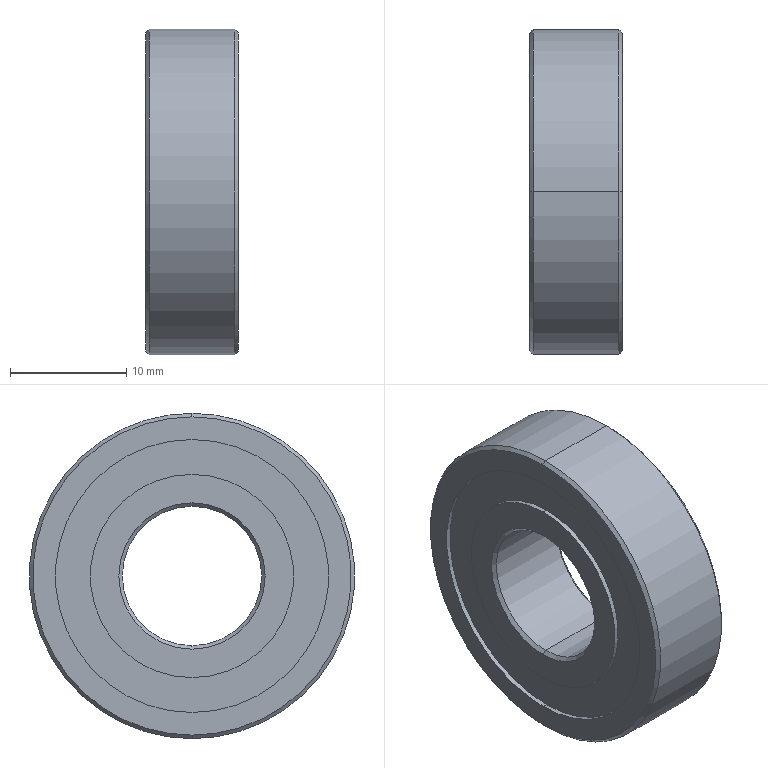Part | SolidWorks | features RefAxis 3, 3DProfileFeature 1, Revolution 1 | 1 solid | 26 faces | box 8 x 28 x 28 mm | volume 3855 mm3 | cylinder 12 | cone 8 | plane 6 | commonest cylinder face diameters 17.5 x4 23.5 x4 12 x2 28 x2
STEP:
#1=CARTESIAN_POINT('',(3.7,0.,14.));
#2=VERTEX_POINT('',#1);
#3=CARTESIAN_POINT('',(3.7,0.,-14.));
#4=VERTEX_POINT('',#3);
#5=CARTESIAN_POINT('',(3.7,0.,0.));
#6=DIRECTION('',(-1.,0.,0.));
#7=DIRECTION('',(0.,0.,1.));
#8=AXIS2_PLACEMENT_3D('',#5,#6,#7);
#9=CIRCLE('',#8,14.);
#10=EDGE_CURVE('',#2,#4,#9,.T.);
#11=ORIENTED_EDGE('',*,*,#10,.T.);
#12=CARTESIAN_POINT('',(-3.7,0.,-14.));
#13=VERTEX_POINT('',#12);
#14=CARTESIAN_POINT('',(4.,0.,-14.));
#15=DIRECTION('',(-1.,0.,0.));
#16=VECTOR('',#15,1000.);
#17=LINE('',#14,#16);
#18=EDGE_CURVE('',#4,#13,#17,.T.);
#19=ORIENTED_EDGE('',*,*,#18,.T.);
#20=CARTESIAN_POINT('',(-3.7,0.,14.));
#21=VERTEX_POINT('',#20);
#22=CARTESIAN_POINT('',(-3.7,0.,0.));
#23=DIRECTION('',(-1.,0.,0.));
#24=DIRECTION('',(0.,0.,1.));
#25=AXIS2_PLACEMENT_3D('',#22,#23,#24);
#26=CIRCLE('',#25,14.);
#27=EDGE_CURVE('',#21,#13,#26,.T.);
#28=ORIENTED_EDGE('',*,*,#27,.F.);
#29=CARTESIAN_POINT('',(4.,0.,14.));
#30=DIRECTION('',(-1.,0.,0.));
#31=VECTOR('',#30,1000.);
#32=LINE('',#29,#31);
#33=EDGE_CURVE('',#2,#21,#32,.T.);
#34=ORIENTED_EDGE('',*,*,#33,.F.);
#35=EDGE_LOOP('',(#11,#19,#28,#34));
#36=FACE_OUTER_BOUND('',#35,.T.);
#37=CARTESIAN_POINT('',(4.,0.,0.));
#38=DIRECTION('',(-1.,0.,0.));
#39=DIRECTION('',(0.,0.,1.));
#40=AXIS2_PLACEMENT_3D('',#37,#38,#39);
#41=CYLINDRICAL_SURFACE('',#40,14.);
#42=ADVANCED_FACE('',(#36),#41,.T.);
#43=CARTESIAN_POINT('',(4.,0.,13.7));
#44=VERTEX_POINT('',#43);
#45=CARTESIAN_POINT('',(4.,0.,-13.7));
#46=VERTEX_POINT('',#45);
#47=CARTESIAN_POINT('',(4.,0.,0.));
#48=DIRECTION('',(-1.,0.,0.));
#49=DIRECTION('',(0.,0.,1.));
#50=AXIS2_PLACEMENT_3D('',#47,#48,#49);
#51=CIRCLE('',#50,13.7);
#52=EDGE_CURVE('',#44,#46,#51,.T.);
#53=ORIENTED_EDGE('',*,*,#52,.T.);
#54=CARTESIAN_POINT('',(4.,0.,-13.7));
#55=DIRECTION('',(-0.7071,0.,-0.7071));
#56=VECTOR('',#55,1000.);
#57=LINE('',#54,#56);
#58=EDGE_CURVE('',#46,#4,#57,.T.);
#59=ORIENTED_EDGE('',*,*,#58,.T.);
#60=ORIENTED_EDGE('',*,*,#10,.F.);
#61=CARTESIAN_POINT('',(4.,0.,13.7));
#62=DIRECTION('',(-0.7071,0.,0.7071));
#63=VECTOR('',#62,1000.);
#64=LINE('',#61,#63);
#65=EDGE_CURVE('',#44,#2,#64,.T.);
#66=ORIENTED_EDGE('',*,*,#65,.F.);
#67=EDGE_LOOP('',(#53,#59,#60,#66));
#68=FACE_OUTER_BOUND('',#67,.T.);
#69=CARTESIAN_POINT('',(4.,0.,0.));
#70=DIRECTION('',(-1.,0.,0.));
#71=DIRECTION('',(0.,0.,1.));
#72=AXIS2_PLACEMENT_3D('',#69,#70,#71);
#73=CONICAL_SURFACE('',#72,13.7,0.7854);
#74=ADVANCED_FACE('',(#68),#73,.T.);
#75=CARTESIAN_POINT('',(4.,0.,-11.75));
#76=VERTEX_POINT('',#75);
#77=CARTESIAN_POINT('',(4.,0.,11.75));
#78=VERTEX_POINT('',#77);
#79=CARTESIAN_POINT('',(4.,0.,0.));
#80=DIRECTION('',(-1.,0.,0.));
#81=DIRECTION('',(0.,0.,1.));
#82=AXIS2_PLACEMENT_3D('',#79,#80,#81);
#83=CIRCLE('',#82,11.75);
#84=EDGE_CURVE('',#76,#78,#83,.T.);
#85=ORIENTED_EDGE('',*,*,#84,.F.);
#86=CARTESIAN_POINT('',(3.6,0.,-11.75));
#87=VERTEX_POINT('',#86);
#88=CARTESIAN_POINT('',(4.,0.,-11.75));
#89=DIRECTION('',(-1.,0.,0.));
#90=VECTOR('',#89,1000.);
#91=LINE('',#88,#90);
#92=EDGE_CURVE('',#76,#87,#91,.T.);
#93=ORIENTED_EDGE('',*,*,#92,.T.);
#94=CARTESIAN_POINT('',(3.6,0.,11.75));
#95=VERTEX_POINT('',#94);
#96=CARTESIAN_POINT('',(3.6,0.,0.));
#97=DIRECTION('',(-1.,0.,0.));
#98=DIRECTION('',(0.,0.,1.));
#99=AXIS2_PLACEMENT_3D('',#96,#97,#98);
#100=CIRCLE('',#99,11.75);
#101=EDGE_CURVE('',#87,#95,#100,.T.);
#102=ORIENTED_EDGE('',*,*,#101,.T.);
#103=CARTESIAN_POINT('',(4.,0.,11.75));
#104=DIRECTION('',(-1.,0.,0.));
#105=VECTOR('',#104,1000.);
#106=LINE('',#103,#105);
#107=EDGE_CURVE('',#78,#95,#106,.T.);
#108=ORIENTED_EDGE('',*,*,#107,.F.);
#109=EDGE_LOOP('',(#85,#93,#102,#108));
#110=FACE_OUTER_BOUND('',#109,.T.);
#111=CARTESIAN_POINT('',(4.,0.,0.));
#112=DIRECTION('',(-1.,0.,0.));
#113=DIRECTION('',(0.,0.,1.));
#114=AXIS2_PLACEMENT_3D('',#111,#112,#113);
#115=CYLINDRICAL_SURFACE('',#114,11.75);
#116=ADVANCED_FACE('',(#110),#115,.F.);
#117=CARTESIAN_POINT('',(4.,0.,8.75));
#118=VERTEX_POINT('',#117);
#119=CARTESIAN_POINT('',(4.,0.,-8.75));
#120=VERTEX_POINT('',#119);
#121=CARTESIAN_POINT('',(4.,0.,0.));
#122=DIRECTION('',(-1.,0.,0.));
#123=DIRECTION('',(0.,0.,1.));
#124=AXIS2_PLACEMENT_3D('',#121,#122,#123);
#125=CIRCLE('',#124,8.75);
#126=EDGE_CURVE('',#118,#120,#125,.T.);
#127=ORIENTED_EDGE('',*,*,#126,.T.);
#128=CARTESIAN_POINT('',(3.6,0.,-8.75));
#129=VERTEX_POINT('',#128);
#130=CARTESIAN_POINT('',(4.,0.,-8.75));
#131=DIRECTION('',(-1.,0.,0.));
#132=VECTOR('',#131,1000.);
#133=LINE('',#130,#132);
#134=EDGE_CURVE('',#120,#129,#133,.T.);
#135=ORIENTED_EDGE('',*,*,#134,.T.);
#136=CARTESIAN_POINT('',(3.6,0.,8.75));
#137=VERTEX_POINT('',#136);
#138=CARTESIAN_POINT('',(3.6,0.,0.));
#139=DIRECTION('',(-1.,0.,0.));
#140=DIRECTION('',(0.,0.,1.));
#141=AXIS2_PLACEMENT_3D('',#138,#139,#140);
#142=CIRCLE('',#141,8.75);
#143=EDGE_CURVE('',#137,#129,#142,.T.);
#144=ORIENTED_EDGE('',*,*,#143,.F.);
#145=CARTESIAN_POINT('',(4.,0.,8.75));
#146=DIRECTION('',(-1.,0.,0.));
#147=VECTOR('',#146,1000.);
#148=LINE('',#145,#147);
#149=EDGE_CURVE('',#118,#137,#148,.T.);
#150=ORIENTED_EDGE('',*,*,#149,.F.);
#151=EDGE_LOOP('',(#127,#135,#144,#150));
#152=FACE_OUTER_BOUND('',#151,.T.);
#153=CARTESIAN_POINT('',(4.,0.,0.));
#154=DIRECTION('',(-1.,0.,0.));
#155=DIRECTION('',(0.,0.,1.));
#156=AXIS2_PLACEMENT_3D('',#153,#154,#155);
#157=CYLINDRICAL_SURFACE('',#156,8.75);
#158=ADVANCED_FACE('',(#152),#157,.T.);
#159=CARTESIAN_POINT('',(3.7,0.,-6.));
#160=VERTEX_POINT('',#159);
#161=CARTESIAN_POINT('',(3.7,0.,6.));
#162=VERTEX_POINT('',#161);
#163=CARTESIAN_POINT('',(3.7,0.,0.));
#164=DIRECTION('',(-1.,0.,0.));
#165=DIRECTION('',(0.,0.,1.));
#166=AXIS2_PLACEMENT_3D('',#163,#164,#165);
#167=CIRCLE('',#166,6.);
#168=EDGE_CURVE('',#160,#162,#167,.T.);
#169=ORIENTED_EDGE('',*,*,#168,.T.);
#170=CARTESIAN_POINT('',(4.,0.,6.3));
#171=VERTEX_POINT('',#170);
#172=CARTESIAN_POINT('',(3.7,0.,6.));
#173=DIRECTION('',(0.7071,0.,0.7071));
#174=VECTOR('',#173,1000.);
#175=LINE('',#172,#174);
#176=EDGE_CURVE('',#162,#171,#175,.T.);
#177=ORIENTED_EDGE('',*,*,#176,.T.);
#178=CARTESIAN_POINT('',(4.,0.,-6.3));
#179=VERTEX_POINT('',#178);
#180=CARTESIAN_POINT('',(4.,0.,0.));
#181=DIRECTION('',(-1.,0.,0.));
#182=DIRECTION('',(0.,0.,1.));
#183=AXIS2_PLACEMENT_3D('',#180,#181,#182);
#184=CIRCLE('',#183,6.3);
#185=EDGE_CURVE('',#179,#171,#184,.T.);
#186=ORIENTED_EDGE('',*,*,#185,.F.);
#187=CARTESIAN_POINT('',(3.7,0.,-6.));
#188=DIRECTION('',(0.7071,0.,-0.7071));
#189=VECTOR('',#188,1000.);
#190=LINE('',#187,#189);
#191=EDGE_CURVE('',#160,#179,#190,.T.);
#192=ORIENTED_EDGE('',*,*,#191,.F.);
#193=EDGE_LOOP('',(#169,#177,#186,#192));
#194=FACE_OUTER_BOUND('',#193,.T.);
#195=CARTESIAN_POINT('',(3.7,0.,0.));
#196=DIRECTION('',(1.,0.,0.));
#197=DIRECTION('',(0.,0.,-1.));
#198=AXIS2_PLACEMENT_3D('',#195,#196,#197);
#199=CONICAL_SURFACE('',#198,6.,0.7854);
#200=ADVANCED_FACE('',(#194),#199,.F.);
#201=ORIENTED_EDGE('',*,*,#168,.F.);
#202=CARTESIAN_POINT('',(-3.7,0.,-6.));
#203=VERTEX_POINT('',#202);
#204=CARTESIAN_POINT('',(4.,0.,-6.));
#205=DIRECTION('',(-1.,0.,0.));
#206=VECTOR('',#205,1000.);
#207=LINE('',#204,#206);
#208=EDGE_CURVE('',#160,#203,#207,.T.);
#209=ORIENTED_EDGE('',*,*,#208,.T.);
#210=CARTESIAN_POINT('',(-3.7,0.,6.));
#211=VERTEX_POINT('',#210);
#212=CARTESIAN_POINT('',(-3.7,0.,0.));
#213=DIRECTION('',(-1.,0.,0.));
#214=DIRECTION('',(0.,0.,1.));
#215=AXIS2_PLACEMENT_3D('',#212,#213,#214);
#216=CIRCLE('',#215,6.);
#217=EDGE_CURVE('',#203,#211,#216,.T.);
#218=ORIENTED_EDGE('',*,*,#217,.T.);
#219=CARTESIAN_POINT('',(4.,0.,6.));
#220=DIRECTION('',(-1.,0.,0.));
#221=VECTOR('',#220,1000.);
#222=LINE('',#219,#221);
#223=EDGE_CURVE('',#162,#211,#222,.T.);
#224=ORIENTED_EDGE('',*,*,#223,.F.);
#225=EDGE_LOOP('',(#201,#209,#218,#224));
#226=FACE_OUTER_BOUND('',#225,.T.);
#227=CARTESIAN_POINT('',(4.,0.,0.));
#228=DIRECTION('',(-1.,0.,0.));
#229=DIRECTION('',(0.,0.,1.));
#230=AXIS2_PLACEMENT_3D('',#227,#228,#229);
#231=CYLINDRICAL_SURFACE('',#230,6.);
#232=ADVANCED_FACE('',(#226),#231,.F.);
#233=ORIENTED_EDGE('',*,*,#217,.F.);
#234=CARTESIAN_POINT('',(-4.,0.,-6.3));
#235=VERTEX_POINT('',#234);
#236=CARTESIAN_POINT('',(-4.,0.,-6.3));
#237=DIRECTION('',(-0.7071,0.,-0.7071));
#238=VECTOR('',#237,1000.);
#239=LINE('',#236,#238);
#240=EDGE_CURVE('',#203,#235,#239,.T.);
#241=ORIENTED_EDGE('',*,*,#240,.T.);
#242=CARTESIAN_POINT('',(-4.,0.,6.3));
#243=VERTEX_POINT('',#242);
#244=CARTESIAN_POINT('',(-4.,0.,0.));
#245=DIRECTION('',(-1.,0.,0.));
#246=DIRECTION('',(0.,0.,1.));
#247=AXIS2_PLACEMENT_3D('',#244,#245,#246);
#248=CIRCLE('',#247,6.3);
#249=EDGE_CURVE('',#235,#243,#248,.T.);
#250=ORIENTED_EDGE('',*,*,#249,.T.);
#251=CARTESIAN_POINT('',(-4.,0.,6.3));
#252=DIRECTION('',(-0.7071,0.,0.7071));
#253=VECTOR('',#252,1000.);
#254=LINE('',#251,#253);
#255=EDGE_CURVE('',#211,#243,#254,.T.);
#256=ORIENTED_EDGE('',*,*,#255,.F.);
#257=EDGE_LOOP('',(#233,#241,#250,#256));
#258=FACE_OUTER_BOUND('',#257,.T.);
#259=CARTESIAN_POINT('',(-4.,0.,0.));
#260=DIRECTION('',(-1.,0.,0.));
#261=DIRECTION('',(0.,0.,1.));
#262=AXIS2_PLACEMENT_3D('',#259,#260,#261);
#263=CONICAL_SURFACE('',#262,6.3,0.7854);
#264=ADVANCED_FACE('',(#258),#263,.F.);
#265=CARTESIAN_POINT('',(-3.6,0.,8.75));
#266=VERTEX_POINT('',#265);
#267=CARTESIAN_POINT('',(-3.6,0.,-8.75));
#268=VERTEX_POINT('',#267);
#269=CARTESIAN_POINT('',(-3.6,0.,0.));
#270=DIRECTION('',(-1.,0.,0.));
#271=DIRECTION('',(0.,0.,1.));
#272=AXIS2_PLACEMENT_3D('',#269,#270,#271);
#273=CIRCLE('',#272,8.75);
#274=EDGE_CURVE('',#266,#268,#273,.T.);
#275=ORIENTED_EDGE('',*,*,#274,.T.);
#276=CARTESIAN_POINT('',(-4.,0.,-8.75));
#277=VERTEX_POINT('',#276);
#278=CARTESIAN_POINT('',(4.,0.,-8.75));
#279=DIRECTION('',(-1.,0.,0.));
#280=VECTOR('',#279,1000.);
#281=LINE('',#278,#280);
#282=EDGE_CURVE('',#268,#277,#281,.T.);
#283=ORIENTED_EDGE('',*,*,#282,.T.);
#284=CARTESIAN_POINT('',(-4.,0.,8.75));
#285=VERTEX_POINT('',#284);
#286=CARTESIAN_POINT('',(-4.,0.,0.));
#287=DIRECTION('',(-1.,0.,0.));
#288=DIRECTION('',(0.,0.,1.));
#289=AXIS2_PLACEMENT_3D('',#286,#287,#288);
#290=CIRCLE('',#289,8.75);
#291=EDGE_CURVE('',#285,#277,#290,.T.);
#292=ORIENTED_EDGE('',*,*,#291,.F.);
#293=CARTESIAN_POINT('',(4.,0.,8.75));
#294=DIRECTION('',(-1.,0.,0.));
#295=VECTOR('',#294,1000.);
#296=LINE('',#293,#295);
#297=EDGE_CURVE('',#266,#285,#296,.T.);
#298=ORIENTED_EDGE('',*,*,#297,.F.);
#299=EDGE_LOOP('',(#275,#283,#292,#298));
#300=FACE_OUTER_BOUND('',#299,.T.);
#301=CARTESIAN_POINT('',(4.,0.,0.));
#302=DIRECTION('',(-1.,0.,0.));
#303=DIRECTION('',(0.,0.,1.));
#304=AXIS2_PLACEMENT_3D('',#301,#302,#303);
#305=CYLINDRICAL_SURFACE('',#304,8.75);
#306=ADVANCED_FACE('',(#300),#305,.T.);
#307=CARTESIAN_POINT('',(-3.6,0.,-11.75));
#308=VERTEX_POINT('',#307);
#309=CARTESIAN_POINT('',(-3.6,0.,11.75));
#310=VERTEX_POINT('',#309);
#311=CARTESIAN_POINT('',(-3.6,0.,0.));
#312=DIRECTION('',(-1.,0.,0.));
#313=DIRECTION('',(0.,0.,1.));
#314=AXIS2_PLACEMENT_3D('',#311,#312,#313);
#315=CIRCLE('',#314,11.75);
#316=EDGE_CURVE('',#308,#310,#315,.T.);
#317=ORIENTED_EDGE('',*,*,#316,.F.);
#318=CARTESIAN_POINT('',(-4.,0.,-11.75));
#319=VERTEX_POINT('',#318);
#320=CARTESIAN_POINT('',(4.,0.,-11.75));
#321=DIRECTION('',(-1.,0.,0.));
#322=VECTOR('',#321,1000.);
#323=LINE('',#320,#322);
#324=EDGE_CURVE('',#308,#319,#323,.T.);
#325=ORIENTED_EDGE('',*,*,#324,.T.);
#326=CARTESIAN_POINT('',(-4.,0.,11.75));
#327=VERTEX_POINT('',#326);
#328=CARTESIAN_POINT('',(-4.,0.,0.));
#329=DIRECTION('',(-1.,0.,0.));
#330=DIRECTION('',(0.,0.,1.));
#331=AXIS2_PLACEMENT_3D('',#328,#329,#330);
#332=CIRCLE('',#331,11.75);
#333=EDGE_CURVE('',#319,#327,#332,.T.);
#334=ORIENTED_EDGE('',*,*,#333,.T.);
#335=CARTESIAN_POINT('',(4.,0.,11.75));
#336=DIRECTION('',(-1.,0.,0.));
#337=VECTOR('',#336,1000.);
#338=LINE('',#335,#337);
#339=EDGE_CURVE('',#310,#327,#338,.T.);
#340=ORIENTED_EDGE('',*,*,#339,.F.);
#341=EDGE_LOOP('',(#317,#325,#334,#340));
#342=FACE_OUTER_BOUND('',#341,.T.);
#343=CARTESIAN_POINT('',(4.,0.,0.));
#344=DIRECTION('',(-1.,0.,0.));
#345=DIRECTION('',(0.,0.,1.));
#346=AXIS2_PLACEMENT_3D('',#343,#344,#345);
#347=CYLINDRICAL_SURFACE('',#346,11.75);
#348=ADVANCED_FACE('',(#342),#347,.F.);
#349=CARTESIAN_POINT('',(-4.,0.,13.7));
#350=VERTEX_POINT('',#349);
#351=CARTESIAN_POINT('',(-4.,0.,-13.7));
#352=VERTEX_POINT('',#351);
#353=CARTESIAN_POINT('',(-4.,0.,0.));
#354=DIRECTION('',(-1.,0.,0.));
#355=DIRECTION('',(0.,0.,1.));
#356=AXIS2_PLACEMENT_3D('',#353,#354,#355);
#357=CIRCLE('',#356,13.7);
#358=EDGE_CURVE('',#350,#352,#357,.T.);
#359=ORIENTED_EDGE('',*,*,#358,.F.);
#360=CARTESIAN_POINT('',(-3.7,0.,14.));
#361=DIRECTION('',(0.7071,0.,0.7071));
#362=VECTOR('',#361,1000.);
#363=LINE('',#360,#362);
#364=EDGE_CURVE('',#350,#21,#363,.T.);
#365=ORIENTED_EDGE('',*,*,#364,.T.);
#366=ORIENTED_EDGE('',*,*,#27,.T.);
#367=CARTESIAN_POINT('',(-3.7,0.,-14.));
#368=DIRECTION('',(0.7071,0.,-0.7071));
#369=VECTOR('',#368,1000.);
#370=LINE('',#367,#369);
#371=EDGE_CURVE('',#352,#13,#370,.T.);
#372=ORIENTED_EDGE('',*,*,#371,.F.);
#373=EDGE_LOOP('',(#359,#365,#366,#372));
#374=FACE_OUTER_BOUND('',#373,.T.);
#375=CARTESIAN_POINT('',(-3.7,0.,0.));
#376=DIRECTION('',(1.,0.,0.));
#377=DIRECTION('',(0.,0.,-1.));
#378=AXIS2_PLACEMENT_3D('',#375,#376,#377);
#379=CONICAL_SURFACE('',#378,14.,0.7854);
#380=ADVANCED_FACE('',(#374),#379,.T.);
#381=ORIENTED_EDGE('',*,*,#364,.F.);
#382=CARTESIAN_POINT('',(-4.,0.,0.));
#383=DIRECTION('',(-1.,0.,0.));
#384=DIRECTION('',(0.,0.,1.));
#385=AXIS2_PLACEMENT_3D('',#382,#383,#384);
#386=CIRCLE('',#385,13.7);
#387=EDGE_CURVE('',#352,#350,#386,.T.);
#388=ORIENTED_EDGE('',*,*,#387,.F.);
#389=ORIENTED_EDGE('',*,*,#371,.T.);
#390=CARTESIAN_POINT('',(-3.7,0.,0.));
#391=DIRECTION('',(-1.,0.,0.));
#392=DIRECTION('',(0.,0.,1.));
#393=AXIS2_PLACEMENT_3D('',#390,#391,#392);
#394=CIRCLE('',#393,14.);
#395=EDGE_CURVE('',#13,#21,#394,.T.);
#396=ORIENTED_EDGE('',*,*,#395,.T.);
#397=EDGE_LOOP('',(#381,#388,#389,#396));
#398=FACE_OUTER_BOUND('',#397,.T.);
#399=CARTESIAN_POINT('',(-3.7,0.,0.));
#400=DIRECTION('',(1.,0.,0.));
#401=DIRECTION('',(0.,0.,-1.));
#402=AXIS2_PLACEMENT_3D('',#399,#400,#401);
#403=CONICAL_SURFACE('',#402,14.,0.7854);
#404=ADVANCED_FACE('',(#398),#403,.T.);
#405=CARTESIAN_POINT('',(-4.,0.,0.));
#406=DIRECTION('',(-1.,0.,0.));
#407=DIRECTION('',(0.,0.,1.));
#408=AXIS2_PLACEMENT_3D('',#405,#406,#407);
#409=CIRCLE('',#408,11.75);
#410=EDGE_CURVE('',#327,#319,#409,.T.);
#411=ORIENTED_EDGE('',*,*,#410,.F.);
#412=ORIENTED_EDGE('',*,*,#333,.F.);
#413=EDGE_LOOP('',(#411,#412));
#414=FACE_BOUND('',#413,.T.);
#415=ORIENTED_EDGE('',*,*,#387,.T.);
#416=ORIENTED_EDGE('',*,*,#358,.T.);
#417=EDGE_LOOP('',(#415,#416));
#418=FACE_OUTER_BOUND('',#417,.T.);
#419=CARTESIAN_POINT('',(-4.,13.7,0.));
#420=DIRECTION('',(1.,0.,0.));
#421=DIRECTION('',(0.,0.,-1.));
#422=AXIS2_PLACEMENT_3D('',#419,#420,#421);
#423=PLANE('',#422);
#424=ADVANCED_FACE('',(#414,#418),#423,.F.);
#425=ORIENTED_EDGE('',*,*,#324,.F.);
#426=CARTESIAN_POINT('',(-3.6,0.,0.));
#427=DIRECTION('',(-1.,0.,0.));
#428=DIRECTION('',(0.,0.,1.));
#429=AXIS2_PLACEMENT_3D('',#426,#427,#428);
#430=CIRCLE('',#429,11.75);
#431=EDGE_CURVE('',#310,#308,#430,.T.);
#432=ORIENTED_EDGE('',*,*,#431,.F.);
#433=ORIENTED_EDGE('',*,*,#339,.T.);
#434=ORIENTED_EDGE('',*,*,#410,.T.);
#435=EDGE_LOOP('',(#425,#432,#433,#434));
#436=FACE_OUTER_BOUND('',#435,.T.);
#437=CARTESIAN_POINT('',(4.,0.,0.));
#438=DIRECTION('',(-1.,0.,0.));
#439=DIRECTION('',(0.,0.,1.));
#440=AXIS2_PLACEMENT_3D('',#437,#438,#439);
#441=CYLINDRICAL_SURFACE('',#440,11.75);
#442=ADVANCED_FACE('',(#436),#441,.F.);
#443=ORIENTED_EDGE('',*,*,#274,.F.);
#444=CARTESIAN_POINT('',(-3.6,0.,0.));
#445=DIRECTION('',(-1.,0.,0.));
#446=DIRECTION('',(0.,0.,1.));
#447=AXIS2_PLACEMENT_3D('',#444,#445,#446);
#448=CIRCLE('',#447,8.75);
#449=EDGE_CURVE('',#268,#266,#448,.T.);
#450=ORIENTED_EDGE('',*,*,#449,.F.);
#451=EDGE_LOOP('',(#443,#450));
#452=FACE_BOUND('',#451,.T.);
#453=ORIENTED_EDGE('',*,*,#431,.T.);
#454=ORIENTED_EDGE('',*,*,#316,.T.);
#455=EDGE_LOOP('',(#453,#454));
#456=FACE_OUTER_BOUND('',#455,.T.);
#457=CARTESIAN_POINT('',(-3.6,11.75,0.));
#458=DIRECTION('',(1.,0.,0.));
#459=DIRECTION('',(0.,0.,-1.));
#460=AXIS2_PLACEMENT_3D('',#457,#458,#459);
#461=PLANE('',#460);
#462=ADVANCED_FACE('',(#452,#456),#461,.F.);
#463=ORIENTED_EDGE('',*,*,#282,.F.);
#464=ORIENTED_EDGE('',*,*,#449,.T.);
#465=ORIENTED_EDGE('',*,*,#297,.T.);
#466=CARTESIAN_POINT('',(-4.,0.,0.));
#467=DIRECTION('',(-1.,0.,0.));
#468=DIRECTION('',(0.,0.,1.));
#469=AXIS2_PLACEMENT_3D('',#466,#467,#468);
#470=CIRCLE('',#469,8.75);
#471=EDGE_CURVE('',#277,#285,#470,.T.);
#472=ORIENTED_EDGE('',*,*,#471,.F.);
#473=EDGE_LOOP('',(#463,#464,#465,#472));
#474=FACE_OUTER_BOUND('',#473,.T.);
#475=CARTESIAN_POINT('',(4.,0.,0.));
#476=DIRECTION('',(-1.,0.,0.));
#477=DIRECTION('',(0.,0.,1.));
#478=AXIS2_PLACEMENT_3D('',#475,#476,#477);
#479=CYLINDRICAL_SURFACE('',#478,8.75);
#480=ADVANCED_FACE('',(#474),#479,.T.);
#481=CARTESIAN_POINT('',(-4.,0.,0.));
#482=DIRECTION('',(-1.,0.,0.));
#483=DIRECTION('',(0.,0.,1.));
#484=AXIS2_PLACEMENT_3D('',#481,#482,#483);
#485=CIRCLE('',#484,6.3);
#486=EDGE_CURVE('',#243,#235,#485,.T.);
#487=ORIENTED_EDGE('',*,*,#486,.F.);
#488=ORIENTED_EDGE('',*,*,#249,.F.);
#489=EDGE_LOOP('',(#487,#488));
#490=FACE_BOUND('',#489,.T.);
#491=ORIENTED_EDGE('',*,*,#291,.T.);
#492=ORIENTED_EDGE('',*,*,#471,.T.);
#493=EDGE_LOOP('',(#491,#492));
#494=FACE_OUTER_BOUND('',#493,.T.);
#495=CARTESIAN_POINT('',(-4.,8.75,0.));
#496=DIRECTION('',(1.,0.,0.));
#497=DIRECTION('',(0.,0.,-1.));
#498=AXIS2_PLACEMENT_3D('',#495,#496,#497);
#499=PLANE('',#498);
#500=ADVANCED_FACE('',(#490,#494),#499,.F.);
#501=ORIENTED_EDGE('',*,*,#240,.F.);
#502=CARTESIAN_POINT('',(-3.7,0.,0.));
#503=DIRECTION('',(-1.,0.,0.));
#504=DIRECTION('',(0.,0.,1.));
#505=AXIS2_PLACEMENT_3D('',#502,#503,#504);
#506=CIRCLE('',#505,6.);
#507=EDGE_CURVE('',#211,#203,#506,.T.);
#508=ORIENTED_EDGE('',*,*,#507,.F.);
#509=ORIENTED_EDGE('',*,*,#255,.T.);
#510=ORIENTED_EDGE('',*,*,#486,.T.);
#511=EDGE_LOOP('',(#501,#508,#509,#510));
#512=FACE_OUTER_BOUND('',#511,.T.);
#513=CARTESIAN_POINT('',(-4.,0.,0.));
#514=DIRECTION('',(-1.,0.,0.));
#515=DIRECTION('',(0.,0.,1.));
#516=AXIS2_PLACEMENT_3D('',#513,#514,#515);
#517=CONICAL_SURFACE('',#516,6.3,0.7854);
#518=ADVANCED_FACE('',(#512),#517,.F.);
#519=ORIENTED_EDGE('',*,*,#208,.F.);
#520=CARTESIAN_POINT('',(3.7,0.,0.));
#521=DIRECTION('',(-1.,0.,0.));
#522=DIRECTION('',(0.,0.,1.));
#523=AXIS2_PLACEMENT_3D('',#520,#521,#522);
#524=CIRCLE('',#523,6.);
#525=EDGE_CURVE('',#162,#160,#524,.T.);
#526=ORIENTED_EDGE('',*,*,#525,.F.);
#527=ORIENTED_EDGE('',*,*,#223,.T.);
#528=ORIENTED_EDGE('',*,*,#507,.T.);
#529=EDGE_LOOP('',(#519,#526,#527,#528));
#530=FACE_OUTER_BOUND('',#529,.T.);
#531=CARTESIAN_POINT('',(4.,0.,0.));
#532=DIRECTION('',(-1.,0.,0.));
#533=DIRECTION('',(0.,0.,1.));
#534=AXIS2_PLACEMENT_3D('',#531,#532,#533);
#535=CYLINDRICAL_SURFACE('',#534,6.);
#536=ADVANCED_FACE('',(#530),#535,.F.);
#537=ORIENTED_EDGE('',*,*,#176,.F.);
#538=ORIENTED_EDGE('',*,*,#525,.T.);
#539=ORIENTED_EDGE('',*,*,#191,.T.);
#540=CARTESIAN_POINT('',(4.,0.,0.));
#541=DIRECTION('',(-1.,0.,0.));
#542=DIRECTION('',(0.,0.,1.));
#543=AXIS2_PLACEMENT_3D('',#540,#541,#542);
#544=CIRCLE('',#543,6.3);
#545=EDGE_CURVE('',#171,#179,#544,.T.);
#546=ORIENTED_EDGE('',*,*,#545,.F.);
#547=EDGE_LOOP('',(#537,#538,#539,#546));
#548=FACE_OUTER_BOUND('',#547,.T.);
#549=CARTESIAN_POINT('',(3.7,0.,0.));
#550=DIRECTION('',(1.,0.,0.));
#551=DIRECTION('',(0.,0.,-1.));
#552=AXIS2_PLACEMENT_3D('',#549,#550,#551);
#553=CONICAL_SURFACE('',#552,6.,0.7854);
#554=ADVANCED_FACE('',(#548),#553,.F.);
#555=ORIENTED_EDGE('',*,*,#126,.F.);
#556=CARTESIAN_POINT('',(4.,0.,0.));
#557=DIRECTION('',(-1.,0.,0.));
#558=DIRECTION('',(0.,0.,1.));
#559=AXIS2_PLACEMENT_3D('',#556,#557,#558);
#560=CIRCLE('',#559,8.75);
#561=EDGE_CURVE('',#120,#118,#560,.T.);
#562=ORIENTED_EDGE('',*,*,#561,.F.);
#563=EDGE_LOOP('',(#555,#562));
#564=FACE_OUTER_BOUND('',#563,.T.);
#565=ORIENTED_EDGE('',*,*,#185,.T.);
#566=ORIENTED_EDGE('',*,*,#545,.T.);
#567=EDGE_LOOP('',(#565,#566));
#568=FACE_BOUND('',#567,.T.);
#569=CARTESIAN_POINT('',(4.,6.3,0.));
#570=DIRECTION('',(-1.,0.,0.));
#571=DIRECTION('',(0.,0.,1.));
#572=AXIS2_PLACEMENT_3D('',#569,#570,#571);
#573=PLANE('',#572);
#574=ADVANCED_FACE('',(#564,#568),#573,.F.);
#575=ORIENTED_EDGE('',*,*,#134,.F.);
#576=ORIENTED_EDGE('',*,*,#561,.T.);
#577=ORIENTED_EDGE('',*,*,#149,.T.);
#578=CARTESIAN_POINT('',(3.6,0.,0.));
#579=DIRECTION('',(-1.,0.,0.));
#580=DIRECTION('',(0.,0.,1.));
#581=AXIS2_PLACEMENT_3D('',#578,#579,#580);
#582=CIRCLE('',#581,8.75);
#583=EDGE_CURVE('',#129,#137,#582,.T.);
#584=ORIENTED_EDGE('',*,*,#583,.F.);
#585=EDGE_LOOP('',(#575,#576,#577,#584));
#586=FACE_OUTER_BOUND('',#585,.T.);
#587=CARTESIAN_POINT('',(4.,0.,0.));
#588=DIRECTION('',(-1.,0.,0.));
#589=DIRECTION('',(0.,0.,1.));
#590=AXIS2_PLACEMENT_3D('',#587,#588,#589);
#591=CYLINDRICAL_SURFACE('',#590,8.75);
#592=ADVANCED_FACE('',(#586),#591,.T.);
#593=CARTESIAN_POINT('',(3.6,0.,0.));
#594=DIRECTION('',(-1.,0.,0.));
#595=DIRECTION('',(0.,0.,1.));
#596=AXIS2_PLACEMENT_3D('',#593,#594,#595);
#597=CIRCLE('',#596,11.75);
#598=EDGE_CURVE('',#95,#87,#597,.T.);
#599=ORIENTED_EDGE('',*,*,#598,.F.);
#600=ORIENTED_EDGE('',*,*,#101,.F.);
#601=EDGE_LOOP('',(#599,#600));
#602=FACE_OUTER_BOUND('',#601,.T.);
#603=ORIENTED_EDGE('',*,*,#143,.T.);
#604=ORIENTED_EDGE('',*,*,#583,.T.);
#605=EDGE_LOOP('',(#603,#604));
#606=FACE_BOUND('',#605,.T.);
#607=CARTESIAN_POINT('',(3.6,8.75,0.));
#608=DIRECTION('',(-1.,0.,0.));
#609=DIRECTION('',(0.,0.,1.));
#610=AXIS2_PLACEMENT_3D('',#607,#608,#609);
#611=PLANE('',#610);
#612=ADVANCED_FACE('',(#602,#606),#611,.F.);
#613=ORIENTED_EDGE('',*,*,#92,.F.);
#614=CARTESIAN_POINT('',(4.,0.,0.));
#615=DIRECTION('',(-1.,0.,0.));
#616=DIRECTION('',(0.,0.,1.));
#617=AXIS2_PLACEMENT_3D('',#614,#615,#616);
#618=CIRCLE('',#617,11.75);
#619=EDGE_CURVE('',#78,#76,#618,.T.);
#620=ORIENTED_EDGE('',*,*,#619,.F.);
#621=ORIENTED_EDGE('',*,*,#107,.T.);
#622=ORIENTED_EDGE('',*,*,#598,.T.);
#623=EDGE_LOOP('',(#613,#620,#621,#622));
#624=FACE_OUTER_BOUND('',#623,.T.);
#625=CARTESIAN_POINT('',(4.,0.,0.));
#626=DIRECTION('',(-1.,0.,0.));
#627=DIRECTION('',(0.,0.,1.));
#628=AXIS2_PLACEMENT_3D('',#625,#626,#627);
#629=CYLINDRICAL_SURFACE('',#628,11.75);
#630=ADVANCED_FACE('',(#624),#629,.F.);
#631=ORIENTED_EDGE('',*,*,#52,.F.);
#632=CARTESIAN_POINT('',(4.,0.,0.));
#633=DIRECTION('',(-1.,0.,0.));
#634=DIRECTION('',(0.,0.,1.));
#635=AXIS2_PLACEMENT_3D('',#632,#633,#634);
#636=CIRCLE('',#635,13.7);
#637=EDGE_CURVE('',#46,#44,#636,.T.);
#638=ORIENTED_EDGE('',*,*,#637,.F.);
#639=EDGE_LOOP('',(#631,#638));
#640=FACE_OUTER_BOUND('',#639,.T.);
#641=ORIENTED_EDGE('',*,*,#619,.T.);
#642=ORIENTED_EDGE('',*,*,#84,.T.);
#643=EDGE_LOOP('',(#641,#642));
#644=FACE_BOUND('',#643,.T.);
#645=CARTESIAN_POINT('',(4.,11.75,0.));
#646=DIRECTION('',(-1.,0.,0.));
#647=DIRECTION('',(0.,0.,1.));
#648=AXIS2_PLACEMENT_3D('',#645,#646,#647);
#649=PLANE('',#648);
#650=ADVANCED_FACE('',(#640,#644),#649,.F.);
#651=ORIENTED_EDGE('',*,*,#58,.F.);
#652=ORIENTED_EDGE('',*,*,#637,.T.);
#653=ORIENTED_EDGE('',*,*,#65,.T.);
#654=CARTESIAN_POINT('',(3.7,0.,0.));
#655=DIRECTION('',(-1.,0.,0.));
#656=DIRECTION('',(0.,0.,1.));
#657=AXIS2_PLACEMENT_3D('',#654,#655,#656);
#658=CIRCLE('',#657,14.);
#659=EDGE_CURVE('',#4,#2,#658,.T.);
#660=ORIENTED_EDGE('',*,*,#659,.F.);
#661=EDGE_LOOP('',(#651,#652,#653,#660));
#662=FACE_OUTER_BOUND('',#661,.T.);
#663=CARTESIAN_POINT('',(4.,0.,0.));
#664=DIRECTION('',(-1.,0.,0.));
#665=DIRECTION('',(0.,0.,1.));
#666=AXIS2_PLACEMENT_3D('',#663,#664,#665);
#667=CONICAL_SURFACE('',#666,13.7,0.7854);
#668=ADVANCED_FACE('',(#662),#667,.T.);
#669=ORIENTED_EDGE('',*,*,#18,.F.);
#670=ORIENTED_EDGE('',*,*,#659,.T.);
#671=ORIENTED_EDGE('',*,*,#33,.T.);
#672=ORIENTED_EDGE('',*,*,#395,.F.);
#673=EDGE_LOOP('',(#669,#670,#671,#672));
#674=FACE_OUTER_BOUND('',#673,.T.);
#675=CARTESIAN_POINT('',(4.,0.,0.));
#676=DIRECTION('',(-1.,0.,0.));
#677=DIRECTION('',(0.,0.,1.));
#678=AXIS2_PLACEMENT_3D('',#675,#676,#677);
#679=CYLINDRICAL_SURFACE('',#678,14.);
#680=ADVANCED_FACE('',(#674),#679,.T.);
#681=CLOSED_SHELL('',(#42,#74,#116,#158,#200,#232,#264,#306,#348,#380,#404,#424,#442,#462,#480,#500,#518,#536,#554,#574,#592,#612,#630,#650,#668,#680));
#682=MANIFOLD_SOLID_BREP('',#681);
#683=CARTESIAN_POINT('',(0.,0.,0.));
#684=DIRECTION('',(0.,0.,1.));
#685=DIRECTION('',(1.,0.,0.));
#686=AXIS2_PLACEMENT_3D('',#683,#684,#685);
#687=(LENGTH_UNIT()NAMED_UNIT(*)SI_UNIT(.MILLI.,.METRE.));
#688=UNCERTAINTY_MEASURE_WITH_UNIT(LENGTH_MEASURE(0.00001),#687,'','');
#689=(NAMED_UNIT(*)PLANE_ANGLE_UNIT()SI_UNIT($,.RADIAN.));
#690=(NAMED_UNIT(*)SI_UNIT($,.STERADIAN.)SOLID_ANGLE_UNIT());
#691=(GEOMETRIC_REPRESENTATION_CONTEXT(3)GLOBAL_UNCERTAINTY_ASSIGNED_CONTEXT((#688))GLOBAL_UNIT_ASSIGNED_CONTEXT((#687,#689,#690))REPRESENTATION_CONTEXT('',''));
#692=ADVANCED_BREP_SHAPE_REPRESENTATION('',(#682,#686),#691);